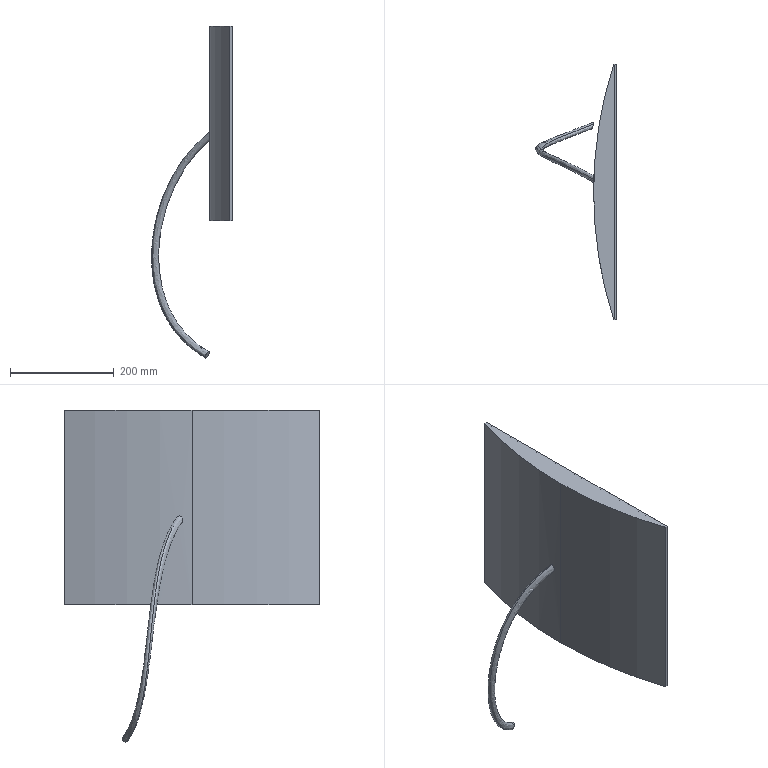Part | SolidWorks | features 3DProfileFeature 2, Extrusion 1, ICE 1, Sweep 1 | 1 solid | 15 faces | box 155.98 x 493 x 640.45 mm | volume 5277382 mm3 | plane 11 | spline 2 | cylinder 2 | commonest cylinder face diameters 1600 x2
STEP:
#1=CARTESIAN_POINT('',(-799.608,25.039,-32.684));
#2=VERTEX_POINT('',#1);
#3=CARTESIAN_POINT('',(-799.627,24.411,-16.43));
#4=VERTEX_POINT('',#3);
#5=CARTESIAN_POINT('',(-799.608,25.039,-32.684));
#6=CARTESIAN_POINT('',(-799.623,24.547,-32.674));
#7=CARTESIAN_POINT('',(-799.638,24.071,-32.597));
#8=CARTESIAN_POINT('',(-799.665,23.143,-32.327));
#9=CARTESIAN_POINT('',(-799.678,22.688,-32.13));
#10=CARTESIAN_POINT('',(-799.696,22.055,-31.769));
#11=CARTESIAN_POINT('',(-799.702,21.851,-31.637));
#12=CARTESIAN_POINT('',(-799.712,21.455,-31.352));
#13=CARTESIAN_POINT('',(-799.717,21.264,-31.198));
#14=CARTESIAN_POINT('',(-799.732,20.715,-30.713));
#15=CARTESIAN_POINT('',(-799.74,20.384,-30.358));
#16=CARTESIAN_POINT('',(-799.755,19.781,-29.594));
#17=CARTESIAN_POINT('',(-799.762,19.51,-29.183));
#18=CARTESIAN_POINT('',(-799.773,19.039,-28.334));
#19=CARTESIAN_POINT('',(-799.778,18.837,-27.894));
#20=CARTESIAN_POINT('',(-799.784,18.582,-27.209));
#21=CARTESIAN_POINT('',(-799.786,18.505,-26.976));
#22=CARTESIAN_POINT('',(-799.789,18.368,-26.508));
#23=CARTESIAN_POINT('',(-799.79,18.309,-26.273));
#24=CARTESIAN_POINT('',(-799.794,18.156,-25.563));
#25=CARTESIAN_POINT('',(-799.795,18.088,-25.085));
#26=CARTESIAN_POINT('',(-799.797,18.022,-24.117));
#27=CARTESIAN_POINT('',(-799.797,18.025,-23.624));
#28=CARTESIAN_POINT('',(-799.795,18.104,-22.659));
#29=CARTESIAN_POINT('',(-799.793,18.179,-22.183));
#30=CARTESIAN_POINT('',(-799.789,18.351,-21.481));
#31=CARTESIAN_POINT('',(-799.788,18.418,-21.248));
#32=CARTESIAN_POINT('',(-799.784,18.573,-20.788));
#33=CARTESIAN_POINT('',(-799.782,18.661,-20.558));
#34=CARTESIAN_POINT('',(-799.775,18.956,-19.887));
#35=CARTESIAN_POINT('',(-799.77,19.191,-19.463));
#36=CARTESIAN_POINT('',(-799.756,19.746,-18.666));
#37=CARTESIAN_POINT('',(-799.748,20.07,-18.29));
#38=CARTESIAN_POINT('',(-799.73,20.783,-17.636));
#39=CARTESIAN_POINT('',(-799.72,21.173,-17.351));
#40=CARTESIAN_POINT('',(-799.703,21.816,-16.999));
#41=CARTESIAN_POINT('',(-799.696,22.04,-16.894));
#42=CARTESIAN_POINT('',(-799.684,22.493,-16.717));
#43=CARTESIAN_POINT('',(-799.677,22.724,-16.644));
#44=CARTESIAN_POINT('',(-799.664,23.194,-16.529));
#45=CARTESIAN_POINT('',(-799.657,23.434,-16.487));
#46=CARTESIAN_POINT('',(-799.642,23.922,-16.434));
#47=CARTESIAN_POINT('',(-799.635,24.168,-16.424));
#48=CARTESIAN_POINT('',(-799.627,24.411,-16.43));
#49=B_SPLINE_CURVE_WITH_KNOTS('',3,(#5,#6,#7,#8,#9,#10,#11,#12,#13,#14,#15,#16,#17,#18,#19,#20,#21,#22,#23,#24,#25,#26,#27,#28,#29,#30,#31,#32,#33,#34,#35,#36,#37,#38,#39,#40,#41,#42,#43,#44,#45,#46,#47,#48),.UNSPECIFIED.,.F.,.F.,(4,2,2,2,2,2,2,2,2,2,2,2,2,2,2,2,2,2,2,2,2,4),(0.,0.001447,0.002894,0.003618,0.004341,0.005789,0.007236,0.008683,0.009407,0.01013,0.01158,0.01302,0.01447,0.0152,0.01592,0.01737,0.01881,0.02026,0.02098,0.02171,0.02243,0.02315),.UNSPECIFIED.);
#50=EDGE_CURVE('',#2,#4,#49,.T.);
#51=ORIENTED_EDGE('',*,*,#50,.T.);
#52=CARTESIAN_POINT('',(-808.512,124.272,-450.652));
#53=VERTEX_POINT('',#52);
#54=CARTESIAN_POINT('',(-799.627,24.411,-16.43));
#55=CARTESIAN_POINT('',(-804.722,27.259,-20.216));
#56=CARTESIAN_POINT('',(-809.675,29.945,-24.241));
#57=CARTESIAN_POINT('',(-831.242,41.331,-43.303));
#58=CARTESIAN_POINT('',(-846.186,48.341,-60.795));
#59=CARTESIAN_POINT('',(-871.819,59.64,-99.448));
#60=CARTESIAN_POINT('',(-882.507,63.928,-120.607));
#61=CARTESIAN_POINT('',(-899.096,70.859,-164.921));
#62=CARTESIAN_POINT('',(-904.996,73.508,-188.073));
#63=CARTESIAN_POINT('',(-911.604,78.299,-234.737));
#64=CARTESIAN_POINT('',(-912.321,80.444,-258.248));
#65=CARTESIAN_POINT('',(-908.19,85.248,-304.097));
#66=CARTESIAN_POINT('',(-903.345,87.902,-326.441));
#67=CARTESIAN_POINT('',(-887.526,94.67,-368.458));
#68=CARTESIAN_POINT('',(-876.545,98.783,-388.138));
#69=CARTESIAN_POINT('',(-847.769,109.451,-423.139));
#70=CARTESIAN_POINT('',(-829.967,116.01,-438.451));
#71=CARTESIAN_POINT('',(-808.512,124.272,-450.652));
#72=B_SPLINE_CURVE_WITH_KNOTS('',3,(#54,#55,#56,#57,#58,#59,#60,#61,#62,#63,#64,#65,#66,#67,#68,#69,#70,#71),.UNSPECIFIED.,.F.,.F.,(4,2,2,2,2,2,2,2,4),(0.08918,0.125,0.25,0.375,0.5,0.625,0.75,0.875,1.),.UNSPECIFIED.);
#73=EDGE_CURVE('',#4,#53,#72,.T.);
#74=ORIENTED_EDGE('',*,*,#73,.T.);
#75=CARTESIAN_POINT('',(-800.416,131.734,-441.656));
#76=VERTEX_POINT('',#75);
#77=CARTESIAN_POINT('',(-804.464,128.003,-446.154));
#78=DIRECTION('',(-0.8213,0.3311,0.4645));
#79=DIRECTION('',(0.5694,0.5248,0.6327));
#80=AXIS2_PLACEMENT_3D('',#77,#78,#79);
#81=CIRCLE('',#80,7.109);
#82=EDGE_CURVE('',#53,#76,#81,.T.);
#83=ORIENTED_EDGE('',*,*,#82,.T.);
#84=CARTESIAN_POINT('',(-799.608,25.039,-32.684));
#85=CARTESIAN_POINT('',(-803.249,27.142,-35.657));
#86=CARTESIAN_POINT('',(-806.805,29.16,-38.765));
#87=CARTESIAN_POINT('',(-825.692,39.703,-56.371));
#88=CARTESIAN_POINT('',(-839.388,46.723,-73.249));
#89=CARTESIAN_POINT('',(-862.835,58.561,-110.495));
#90=CARTESIAN_POINT('',(-872.581,63.381,-130.861));
#91=CARTESIAN_POINT('',(-887.671,71.722,-173.447));
#92=CARTESIAN_POINT('',(-893.02,75.241,-195.663));
#93=CARTESIAN_POINT('',(-898.915,81.744,-240.318));
#94=CARTESIAN_POINT('',(-899.46,84.72,-262.756));
#95=CARTESIAN_POINT('',(-895.258,90.915,-306.258));
#96=CARTESIAN_POINT('',(-890.509,94.135,-327.318));
#97=CARTESIAN_POINT('',(-875.251,101.738,-366.523));
#98=CARTESIAN_POINT('',(-864.752,106.121,-384.668));
#99=CARTESIAN_POINT('',(-837.484,117.041,-416.692));
#100=CARTESIAN_POINT('',(-820.713,123.579,-430.585));
#101=CARTESIAN_POINT('',(-800.416,131.734,-441.656));
#102=B_SPLINE_CURVE_WITH_KNOTS('',3,(#84,#85,#86,#87,#88,#89,#90,#91,#92,#93,#94,#95,#96,#97,#98,#99,#100,#101),.UNSPECIFIED.,.F.,.F.,(4,2,2,2,2,2,2,2,4),(0.09687,0.125,0.25,0.375,0.5,0.625,0.75,0.875,1.),.UNSPECIFIED.);
#103=EDGE_CURVE('',#2,#76,#102,.T.);
#104=ORIENTED_EDGE('',*,*,#103,.F.);
#105=EDGE_LOOP('',(#51,#74,#83,#104));
#106=FACE_OUTER_BOUND('',#105,.T.);
#107=CARTESIAN_POINT('',(-759.077,0.,-7.109));
#108=CARTESIAN_POINT('',(-777.726,12.299,-15.756));
#109=CARTESIAN_POINT('',(-794.858,22.49,-27.627));
#110=CARTESIAN_POINT('',(-825.692,39.703,-56.371));
#111=CARTESIAN_POINT('',(-839.388,46.723,-73.249));
#112=CARTESIAN_POINT('',(-862.835,58.561,-110.495));
#113=CARTESIAN_POINT('',(-872.581,63.381,-130.861));
#114=CARTESIAN_POINT('',(-887.671,71.722,-173.447));
#115=CARTESIAN_POINT('',(-893.02,75.241,-195.663));
#116=CARTESIAN_POINT('',(-898.915,81.744,-240.318));
#117=CARTESIAN_POINT('',(-899.46,84.72,-262.756));
#118=CARTESIAN_POINT('',(-895.258,90.915,-306.258));
#119=CARTESIAN_POINT('',(-890.509,94.135,-327.318));
#120=CARTESIAN_POINT('',(-875.251,101.738,-366.523));
#121=CARTESIAN_POINT('',(-864.752,106.121,-384.668));
#122=CARTESIAN_POINT('',(-837.484,117.041,-416.692));
#123=CARTESIAN_POINT('',(-820.713,123.579,-430.585));
#124=CARTESIAN_POINT('',(-800.416,131.734,-441.656));
#125=CARTESIAN_POINT('',(-759.077,14.218,-7.109));
#126=CARTESIAN_POINT('',(-778.229,26.518,-16.401));
#127=CARTESIAN_POINT('',(-795.775,36.636,-28.921));
#128=CARTESIAN_POINT('',(-827.363,53.635,-58.761));
#129=CARTESIAN_POINT('',(-841.41,60.52,-76.085));
#130=CARTESIAN_POINT('',(-865.677,72.042,-114.055));
#131=CARTESIAN_POINT('',(-875.9,76.678,-134.703));
#132=CARTESIAN_POINT('',(-892.018,84.529,-177.881));
#133=CARTESIAN_POINT('',(-897.911,87.735,-200.416));
#134=CARTESIAN_POINT('',(-904.625,93.542,-245.868));
#135=CARTESIAN_POINT('',(-905.433,96.143,-268.785));
#136=CARTESIAN_POINT('',(-901.239,101.734,-313.307));
#137=CARTESIAN_POINT('',(-896.235,104.731,-334.905));
#138=CARTESIAN_POINT('',(-879.972,112.146,-375.01));
#139=CARTESIAN_POINT('',(-868.721,116.564,-393.507));
#140=CARTESIAN_POINT('',(-839.746,127.746,-425.815));
#141=CARTESIAN_POINT('',(-822.035,134.503,-439.634));
#142=CARTESIAN_POINT('',(-800.904,142.884,-450.466));
#143=CARTESIAN_POINT('',(-759.077,14.218,7.109));
#144=CARTESIAN_POINT('',(-779.636,27.162,-2.182));
#145=CARTESIAN_POINT('',(-798.632,37.778,-14.965));
#146=CARTESIAN_POINT('',(-832.913,55.263,-45.692));
#147=CARTESIAN_POINT('',(-848.208,62.138,-63.631));
#148=CARTESIAN_POINT('',(-874.661,73.121,-103.007));
#149=CARTESIAN_POINT('',(-885.826,77.224,-124.449));
#150=CARTESIAN_POINT('',(-903.443,83.666,-169.355));
#151=CARTESIAN_POINT('',(-909.887,86.002,-192.826));
#152=CARTESIAN_POINT('',(-917.314,90.097,-240.287));
#153=CARTESIAN_POINT('',(-918.295,91.867,-264.277));
#154=CARTESIAN_POINT('',(-914.172,96.067,-311.146));
#155=CARTESIAN_POINT('',(-909.071,98.498,-334.029));
#156=CARTESIAN_POINT('',(-892.248,105.077,-376.945));
#157=CARTESIAN_POINT('',(-880.515,109.226,-396.976));
#158=CARTESIAN_POINT('',(-850.031,120.155,-432.262));
#159=CARTESIAN_POINT('',(-831.288,126.934,-447.5));
#160=CARTESIAN_POINT('',(-809.,135.421,-459.462));
#161=CARTESIAN_POINT('',(-759.077,0.,7.109));
#162=CARTESIAN_POINT('',(-779.134,12.944,-1.538));
#163=CARTESIAN_POINT('',(-797.715,23.632,-13.671));
#164=CARTESIAN_POINT('',(-831.242,41.331,-43.303));
#165=CARTESIAN_POINT('',(-846.186,48.341,-60.795));
#166=CARTESIAN_POINT('',(-871.819,59.64,-99.448));
#167=CARTESIAN_POINT('',(-882.507,63.928,-120.607));
#168=CARTESIAN_POINT('',(-899.096,70.859,-164.921));
#169=CARTESIAN_POINT('',(-904.996,73.508,-188.073));
#170=CARTESIAN_POINT('',(-911.604,78.299,-234.737));
#171=CARTESIAN_POINT('',(-912.321,80.444,-258.248));
#172=CARTESIAN_POINT('',(-908.19,85.248,-304.097));
#173=CARTESIAN_POINT('',(-903.345,87.902,-326.441));
#174=CARTESIAN_POINT('',(-887.526,94.67,-368.458));
#175=CARTESIAN_POINT('',(-876.545,98.783,-388.138));
#176=CARTESIAN_POINT('',(-847.769,109.451,-423.139));
#177=CARTESIAN_POINT('',(-829.967,116.01,-438.451));
#178=CARTESIAN_POINT('',(-808.512,124.272,-450.652));
#179=CARTESIAN_POINT('',(-759.077,-14.218,7.109));
#180=CARTESIAN_POINT('',(-778.631,-1.274,-0.8927));
#181=CARTESIAN_POINT('',(-796.798,9.486,-12.378));
#182=CARTESIAN_POINT('',(-829.57,27.398,-40.913));
#183=CARTESIAN_POINT('',(-844.163,34.545,-57.958));
#184=CARTESIAN_POINT('',(-868.977,46.159,-95.888));
#185=CARTESIAN_POINT('',(-879.188,50.631,-116.766));
#186=CARTESIAN_POINT('',(-894.749,58.052,-160.487));
#187=CARTESIAN_POINT('',(-900.105,61.014,-183.32));
#188=CARTESIAN_POINT('',(-905.894,66.501,-229.186));
#189=CARTESIAN_POINT('',(-906.348,69.021,-252.219));
#190=CARTESIAN_POINT('',(-902.209,74.429,-297.048));
#191=CARTESIAN_POINT('',(-897.619,77.307,-318.854));
#192=CARTESIAN_POINT('',(-882.805,84.263,-359.972));
#193=CARTESIAN_POINT('',(-872.576,88.34,-379.299));
#194=CARTESIAN_POINT('',(-845.507,98.747,-414.016));
#195=CARTESIAN_POINT('',(-828.645,105.086,-429.402));
#196=CARTESIAN_POINT('',(-808.025,113.123,-441.842));
#197=CARTESIAN_POINT('',(-759.077,-14.218,-7.109));
#198=CARTESIAN_POINT('',(-777.224,-1.919,-15.111));
#199=CARTESIAN_POINT('',(-793.941,8.344,-26.334));
#200=CARTESIAN_POINT('',(-824.02,25.771,-53.981));
#201=CARTESIAN_POINT('',(-837.366,32.927,-70.412));
#202=CARTESIAN_POINT('',(-859.993,45.08,-106.936));
#203=CARTESIAN_POINT('',(-869.262,50.085,-127.02));
#204=CARTESIAN_POINT('',(-883.324,58.915,-169.013));
#205=CARTESIAN_POINT('',(-888.129,62.747,-190.91));
#206=CARTESIAN_POINT('',(-893.205,69.946,-234.767));
#207=CARTESIAN_POINT('',(-893.486,73.297,-256.727));
#208=CARTESIAN_POINT('',(-889.277,80.096,-299.209));
#209=CARTESIAN_POINT('',(-884.782,83.54,-319.73));
#210=CARTESIAN_POINT('',(-870.53,91.331,-358.037));
#211=CARTESIAN_POINT('',(-860.783,95.678,-375.83));
#212=CARTESIAN_POINT('',(-835.222,106.337,-407.569));
#213=CARTESIAN_POINT('',(-819.392,112.655,-421.537));
#214=CARTESIAN_POINT('',(-799.929,120.585,-432.846));
#215=CARTESIAN_POINT('',(-759.077,0.,-7.109));
#216=CARTESIAN_POINT('',(-777.726,12.299,-15.756));
#217=CARTESIAN_POINT('',(-794.858,22.49,-27.627));
#218=CARTESIAN_POINT('',(-825.692,39.703,-56.371));
#219=CARTESIAN_POINT('',(-839.388,46.723,-73.249));
#220=CARTESIAN_POINT('',(-862.835,58.561,-110.495));
#221=CARTESIAN_POINT('',(-872.581,63.381,-130.861));
#222=CARTESIAN_POINT('',(-887.671,71.722,-173.447));
#223=CARTESIAN_POINT('',(-893.02,75.241,-195.663));
#224=CARTESIAN_POINT('',(-898.915,81.744,-240.318));
#225=CARTESIAN_POINT('',(-899.46,84.72,-262.756));
#226=CARTESIAN_POINT('',(-895.258,90.915,-306.258));
#227=CARTESIAN_POINT('',(-890.509,94.135,-327.318));
#228=CARTESIAN_POINT('',(-875.251,101.738,-366.523));
#229=CARTESIAN_POINT('',(-864.752,106.121,-384.668));
#230=CARTESIAN_POINT('',(-837.484,117.041,-416.692));
#231=CARTESIAN_POINT('',(-820.713,123.579,-430.585));
#232=CARTESIAN_POINT('',(-800.416,131.734,-441.656));
#233=(BOUNDED_SURFACE()B_SPLINE_SURFACE(3,3,((#107,#108,#109,#110,#111,#112,#113,#114,#115,#116,#117,#118,#119,#120,#121,#122,#123,#124),(#125,#126,#127,#128,#129,#130,#131,#132,#133,#134,#135,#136,#137,#138,#139,#140,#141,#142),(#143,#144,#145,#146,#147,#148,#149,#150,#151,#152,#153,#154,#155,#156,#157,#158,#159,#160),(#161,#162,#163,#164,#165,#166,#167,#168,#169,#170,#171,#172,#173,#174,#175,#176,#177,#178),(#179,#180,#181,#182,#183,#184,#185,#186,#187,#188,#189,#190,#191,#192,#193,#194,#195,#196),(#197,#198,#199,#200,#201,#202,#203,#204,#205,#206,#207,#208,#209,#210,#211,#212,#213,#214),(#215,#216,#217,#218,#219,#220,#221,#222,#223,#224,#225,#226,#227,#228,#229,#230,#231,#232)),.UNSPECIFIED.,.T.,.F.,.F.)B_SPLINE_SURFACE_WITH_KNOTS((4,3,4),(4,2,2,2,2,2,2,2,4),(0.,0.5,1.),(0.,0.125,0.25,0.375,0.5,0.625,0.75,0.875,1.),.UNSPECIFIED.)GEOMETRIC_REPRESENTATION_ITEM()RATIONAL_B_SPLINE_SURFACE(((1.,1.,1.,1.,1.,1.,1.,1.,1.,1.,1.,1.,1.,1.,1.,1.,1.,1.),(0.3333,0.3333,0.3333,0.3333,0.3333,0.3333,0.3333,0.3333,0.3333,0.3333,0.3333,0.3333,0.3333,0.3333,0.3333,0.3333,0.3333,0.3333),(0.3333,0.3333,0.3333,0.3333,0.3333,0.3333,0.3333,0.3333,0.3333,0.3333,0.3333,0.3333,0.3333,0.3333,0.3333,0.3333,0.3333,0.3333),(1.,1.,1.,1.,1.,1.,1.,1.,1.,1.,1.,1.,1.,1.,1.,1.,1.,1.),(0.3333,0.3333,0.3333,0.3333,0.3333,0.3333,0.3333,0.3333,0.3333,0.3333,0.3333,0.3333,0.3333,0.3333,0.3333,0.3333,0.3333,0.3333),(0.3333,0.3333,0.3333,0.3333,0.3333,0.3333,0.3333,0.3333,0.3333,0.3333,0.3333,0.3333,0.3333,0.3333,0.3333,0.3333,0.3333,0.3333),(1.,1.,1.,1.,1.,1.,1.,1.,1.,1.,1.,1.,1.,1.,1.,1.,1.,1.)))REPRESENTATION_ITEM('')SURFACE());
#234=ADVANCED_FACE('',(#106),#233,.F.);
#235=CARTESIAN_POINT('',(-800.,0.,188.));
#236=VERTEX_POINT('',#235);
#237=CARTESIAN_POINT('',(-761.077,-246.5,188.));
#238=VERTEX_POINT('',#237);
#239=CARTESIAN_POINT('',(0.,0.,188.));
#240=DIRECTION('',(0.,0.,1.));
#241=DIRECTION('',(1.,0.,0.));
#242=AXIS2_PLACEMENT_3D('',#239,#240,#241);
#243=CIRCLE('',#242,800.);
#244=EDGE_CURVE('',#236,#238,#243,.T.);
#245=ORIENTED_EDGE('',*,*,#244,.F.);
#246=CARTESIAN_POINT('',(-800.,0.,-188.));
#247=VERTEX_POINT('',#246);
#248=CARTESIAN_POINT('',(-800.,0.,188.));
#249=DIRECTION('',(0.,0.,-1.));
#250=VECTOR('',#249,1000.);
#251=LINE('',#248,#250);
#252=EDGE_CURVE('',#236,#247,#251,.T.);
#253=ORIENTED_EDGE('',*,*,#252,.T.);
#254=CARTESIAN_POINT('',(-761.077,-246.5,-188.));
#255=VERTEX_POINT('',#254);
#256=CARTESIAN_POINT('',(0.,0.,-188.));
#257=DIRECTION('',(0.,0.,1.));
#258=DIRECTION('',(1.,0.,0.));
#259=AXIS2_PLACEMENT_3D('',#256,#257,#258);
#260=CIRCLE('',#259,800.);
#261=EDGE_CURVE('',#247,#255,#260,.T.);
#262=ORIENTED_EDGE('',*,*,#261,.T.);
#263=CARTESIAN_POINT('',(-761.077,-246.5,188.));
#264=DIRECTION('',(0.,0.,-1.));
#265=VECTOR('',#264,1000.);
#266=LINE('',#263,#265);
#267=EDGE_CURVE('',#238,#255,#266,.T.);
#268=ORIENTED_EDGE('',*,*,#267,.F.);
#269=EDGE_LOOP('',(#245,#253,#262,#268));
#270=FACE_OUTER_BOUND('',#269,.T.);
#271=CARTESIAN_POINT('',(0.,0.,188.));
#272=DIRECTION('',(0.,0.,-1.));
#273=DIRECTION('',(-1.,0.,0.));
#274=AXIS2_PLACEMENT_3D('',#271,#272,#273);
#275=CYLINDRICAL_SURFACE('',#274,800.);
#276=ADVANCED_FACE('',(#270),#275,.T.);
#277=ORIENTED_EDGE('',*,*,#252,.F.);
#278=CARTESIAN_POINT('',(-761.077,246.5,188.));
#279=VERTEX_POINT('',#278);
#280=CARTESIAN_POINT('',(0.,0.,188.));
#281=DIRECTION('',(0.,0.,1.));
#282=DIRECTION('',(1.,0.,0.));
#283=AXIS2_PLACEMENT_3D('',#280,#281,#282);
#284=CIRCLE('',#283,800.);
#285=EDGE_CURVE('',#279,#236,#284,.T.);
#286=ORIENTED_EDGE('',*,*,#285,.F.);
#287=CARTESIAN_POINT('',(-761.077,246.5,-188.));
#288=VERTEX_POINT('',#287);
#289=CARTESIAN_POINT('',(-761.077,246.5,188.));
#290=DIRECTION('',(0.,0.,-1.));
#291=VECTOR('',#290,1000.);
#292=LINE('',#289,#291);
#293=EDGE_CURVE('',#279,#288,#292,.T.);
#294=ORIENTED_EDGE('',*,*,#293,.T.);
#295=CARTESIAN_POINT('',(0.,0.,-188.));
#296=DIRECTION('',(0.,0.,1.));
#297=DIRECTION('',(1.,0.,0.));
#298=AXIS2_PLACEMENT_3D('',#295,#296,#297);
#299=CIRCLE('',#298,800.);
#300=EDGE_CURVE('',#288,#247,#299,.T.);
#301=ORIENTED_EDGE('',*,*,#300,.T.);
#302=EDGE_LOOP('',(#277,#286,#294,#301));
#303=FACE_OUTER_BOUND('',#302,.T.);
#304=ORIENTED_EDGE('',*,*,#50,.F.);
#305=CARTESIAN_POINT('',(-799.627,24.411,-16.43));
#306=CARTESIAN_POINT('',(-799.62,24.653,-16.436));
#307=CARTESIAN_POINT('',(-799.613,24.893,-16.458));
#308=CARTESIAN_POINT('',(-799.598,25.371,-16.531));
#309=CARTESIAN_POINT('',(-799.59,25.611,-16.584));
#310=CARTESIAN_POINT('',(-799.567,26.313,-16.784));
#311=CARTESIAN_POINT('',(-799.552,26.759,-16.971));
#312=CARTESIAN_POINT('',(-799.531,27.396,-17.326));
#313=CARTESIAN_POINT('',(-799.524,27.604,-17.457));
#314=CARTESIAN_POINT('',(-799.51,28.,-17.736));
#315=CARTESIAN_POINT('',(-799.503,28.19,-17.885));
#316=CARTESIAN_POINT('',(-799.484,28.738,-18.361));
#317=CARTESIAN_POINT('',(-799.472,29.076,-18.717));
#318=CARTESIAN_POINT('',(-799.449,29.678,-19.476));
#319=CARTESIAN_POINT('',(-799.439,29.944,-19.879));
#320=CARTESIAN_POINT('',(-799.422,30.412,-20.729));
#321=CARTESIAN_POINT('',(-799.414,30.612,-21.176));
#322=CARTESIAN_POINT('',(-799.401,30.941,-22.084));
#323=CARTESIAN_POINT('',(-799.396,31.07,-22.549));
#324=CARTESIAN_POINT('',(-799.389,31.262,-23.499));
#325=CARTESIAN_POINT('',(-799.387,31.323,-23.985));
#326=CARTESIAN_POINT('',(-799.385,31.375,-24.947));
#327=CARTESIAN_POINT('',(-799.385,31.366,-25.428));
#328=CARTESIAN_POINT('',(-799.388,31.276,-26.389));
#329=CARTESIAN_POINT('',(-799.392,31.194,-26.874));
#330=CARTESIAN_POINT('',(-799.401,30.959,-27.81));
#331=CARTESIAN_POINT('',(-799.407,30.805,-28.264));
#332=CARTESIAN_POINT('',(-799.418,30.518,-28.924));
#333=CARTESIAN_POINT('',(-799.422,30.412,-29.14));
#334=CARTESIAN_POINT('',(-799.431,30.181,-29.564));
#335=CARTESIAN_POINT('',(-799.435,30.053,-29.773));
#336=CARTESIAN_POINT('',(-799.451,29.643,-30.378));
#337=CARTESIAN_POINT('',(-799.462,29.334,-30.75));
#338=CARTESIAN_POINT('',(-799.481,28.809,-31.253));
#339=CARTESIAN_POINT('',(-799.488,28.623,-31.412));
#340=CARTESIAN_POINT('',(-799.502,28.234,-31.706));
#341=CARTESIAN_POINT('',(-799.509,28.032,-31.84));
#342=CARTESIAN_POINT('',(-799.523,27.615,-32.081));
#343=CARTESIAN_POINT('',(-799.531,27.4,-32.187));
#344=CARTESIAN_POINT('',(-799.546,26.954,-32.372));
#345=CARTESIAN_POINT('',(-799.554,26.722,-32.451));
#346=CARTESIAN_POINT('',(-799.577,26.012,-32.637));
#347=CARTESIAN_POINT('',(-799.593,25.528,-32.694));
#348=CARTESIAN_POINT('',(-799.608,25.039,-32.684));
#349=B_SPLINE_CURVE_WITH_KNOTS('',3,(#305,#306,#307,#308,#309,#310,#311,#312,#313,#314,#315,#316,#317,#318,#319,#320,#321,#322,#323,#324,#325,#326,#327,#328,#329,#330,#331,#332,#333,#334,#335,#336,#337,#338,#339,#340,#341,#342,#343,#344,#345,#346,#347,#348),.UNSPECIFIED.,.F.,.F.,(4,2,2,2,2,2,2,2,2,2,2,2,2,2,2,2,2,2,2,2,2,4),(0.02315,0.02387,0.02459,0.02603,0.02675,0.02747,0.02891,0.03034,0.03178,0.03322,0.03466,0.0361,0.03753,0.03897,0.03969,0.04041,0.04185,0.04257,0.04329,0.04401,0.04472,0.04616),.UNSPECIFIED.);
#350=EDGE_CURVE('',#4,#2,#349,.T.);
#351=ORIENTED_EDGE('',*,*,#350,.F.);
#352=EDGE_LOOP('',(#304,#351));
#353=FACE_BOUND('',#352,.T.);
#354=CARTESIAN_POINT('',(0.,0.,188.));
#355=DIRECTION('',(0.,0.,-1.));
#356=DIRECTION('',(-1.,0.,0.));
#357=AXIS2_PLACEMENT_3D('',#354,#355,#356);
#358=CYLINDRICAL_SURFACE('',#357,800.);
#359=ADVANCED_FACE('',(#303,#353),#358,.T.);
#360=CARTESIAN_POINT('',(-756.077,246.5,-188.));
#361=VERTEX_POINT('',#360);
#362=CARTESIAN_POINT('',(0.,246.5,-188.));
#363=DIRECTION('',(-1.,0.,0.));
#364=VECTOR('',#363,1000.);
#365=LINE('',#362,#364);
#366=EDGE_CURVE('',#361,#288,#365,.T.);
#367=ORIENTED_EDGE('',*,*,#366,.T.);
#368=ORIENTED_EDGE('',*,*,#293,.F.);
#369=CARTESIAN_POINT('',(-756.077,246.5,188.));
#370=VERTEX_POINT('',#369);
#371=CARTESIAN_POINT('',(0.,246.5,188.));
#372=DIRECTION('',(-1.,0.,0.));
#373=VECTOR('',#372,1000.);
#374=LINE('',#371,#373);
#375=EDGE_CURVE('',#370,#279,#374,.T.);
#376=ORIENTED_EDGE('',*,*,#375,.F.);
#377=CARTESIAN_POINT('',(-756.077,246.5,188.));
#378=DIRECTION('',(0.,0.,-1.));
#379=VECTOR('',#378,1000.);
#380=LINE('',#377,#379);
#381=EDGE_CURVE('',#370,#361,#380,.T.);
#382=ORIENTED_EDGE('',*,*,#381,.T.);
#383=EDGE_LOOP('',(#367,#368,#376,#382));
#384=FACE_OUTER_BOUND('',#383,.T.);
#385=CARTESIAN_POINT('',(0.,246.5,188.));
#386=DIRECTION('',(0.,-1.,0.));
#387=DIRECTION('',(1.,0.,0.));
#388=AXIS2_PLACEMENT_3D('',#385,#386,#387);
#389=PLANE('',#388);
#390=ADVANCED_FACE('',(#384),#389,.F.);
#391=CARTESIAN_POINT('',(-756.077,-246.5,-188.));
#392=VERTEX_POINT('',#391);
#393=CARTESIAN_POINT('',(0.,-246.5,-188.));
#394=DIRECTION('',(-1.,0.,0.));
#395=VECTOR('',#394,1000.);
#396=LINE('',#393,#395);
#397=EDGE_CURVE('',#392,#255,#396,.T.);
#398=ORIENTED_EDGE('',*,*,#397,.F.);
#399=CARTESIAN_POINT('',(-756.077,-246.5,188.));
#400=VERTEX_POINT('',#399);
#401=CARTESIAN_POINT('',(-756.077,-246.5,188.));
#402=DIRECTION('',(0.,0.,-1.));
#403=VECTOR('',#402,1000.);
#404=LINE('',#401,#403);
#405=EDGE_CURVE('',#400,#392,#404,.T.);
#406=ORIENTED_EDGE('',*,*,#405,.F.);
#407=CARTESIAN_POINT('',(0.,-246.5,188.));
#408=DIRECTION('',(-1.,0.,0.));
#409=VECTOR('',#408,1000.);
#410=LINE('',#407,#409);
#411=EDGE_CURVE('',#400,#238,#410,.T.);
#412=ORIENTED_EDGE('',*,*,#411,.T.);
#413=ORIENTED_EDGE('',*,*,#267,.T.);
#414=EDGE_LOOP('',(#398,#406,#412,#413));
#415=FACE_OUTER_BOUND('',#414,.T.);
#416=CARTESIAN_POINT('',(0.,-246.5,188.));
#417=DIRECTION('',(0.,-1.,0.));
#418=DIRECTION('',(1.,0.,0.));
#419=AXIS2_PLACEMENT_3D('',#416,#417,#418);
#420=PLANE('',#419);
#421=ADVANCED_FACE('',(#415),#420,.T.);
#422=CARTESIAN_POINT('',(-756.077,-244.5,-186.));
#423=VERTEX_POINT('',#422);
#424=CARTESIAN_POINT('',(-756.077,244.5,-186.));
#425=VERTEX_POINT('',#424);
#426=CARTESIAN_POINT('',(-756.077,-244.5,-186.));
#427=DIRECTION('',(0.,1.,0.));
#428=VECTOR('',#427,1000.);
#429=LINE('',#426,#428);
#430=EDGE_CURVE('',#423,#425,#429,.T.);
#431=ORIENTED_EDGE('',*,*,#430,.F.);
#432=CARTESIAN_POINT('',(-756.077,-244.5,186.));
#433=VERTEX_POINT('',#432);
#434=CARTESIAN_POINT('',(-756.077,-244.5,186.));
#435=DIRECTION('',(0.,0.,-1.));
#436=VECTOR('',#435,1000.);
#437=LINE('',#434,#436);
#438=EDGE_CURVE('',#433,#423,#437,.T.);
#439=ORIENTED_EDGE('',*,*,#438,.F.);
#440=CARTESIAN_POINT('',(-756.077,244.5,186.));
#441=VERTEX_POINT('',#440);
#442=CARTESIAN_POINT('',(-756.077,244.5,186.));
#443=DIRECTION('',(0.,-1.,0.));
#444=VECTOR('',#443,1000.);
#445=LINE('',#442,#444);
#446=EDGE_CURVE('',#441,#433,#445,.T.);
#447=ORIENTED_EDGE('',*,*,#446,.F.);
#448=CARTESIAN_POINT('',(-756.077,244.5,-186.));
#449=DIRECTION('',(0.,0.,1.));
#450=VECTOR('',#449,1000.);
#451=LINE('',#448,#450);
#452=EDGE_CURVE('',#425,#441,#451,.T.);
#453=ORIENTED_EDGE('',*,*,#452,.F.);
#454=EDGE_LOOP('',(#431,#439,#447,#453));
#455=FACE_BOUND('',#454,.T.);
#456=CARTESIAN_POINT('',(-756.077,0.,-188.));
#457=DIRECTION('',(0.,1.,0.));
#458=VECTOR('',#457,1000.);
#459=LINE('',#456,#458);
#460=EDGE_CURVE('',#392,#361,#459,.T.);
#461=ORIENTED_EDGE('',*,*,#460,.T.);
#462=ORIENTED_EDGE('',*,*,#381,.F.);
#463=CARTESIAN_POINT('',(-756.077,0.,188.));
#464=DIRECTION('',(0.,1.,0.));
#465=VECTOR('',#464,1000.);
#466=LINE('',#463,#465);
#467=EDGE_CURVE('',#400,#370,#466,.T.);
#468=ORIENTED_EDGE('',*,*,#467,.F.);
#469=ORIENTED_EDGE('',*,*,#405,.T.);
#470=EDGE_LOOP('',(#461,#462,#468,#469));
#471=FACE_OUTER_BOUND('',#470,.T.);
#472=CARTESIAN_POINT('',(-756.077,0.,188.));
#473=DIRECTION('',(-1.,0.,0.));
#474=DIRECTION('',(0.,-1.,0.));
#475=AXIS2_PLACEMENT_3D('',#472,#473,#474);
#476=PLANE('',#475);
#477=ADVANCED_FACE('',(#455,#471),#476,.F.);
#478=ORIENTED_EDGE('',*,*,#375,.T.);
#479=ORIENTED_EDGE('',*,*,#285,.T.);
#480=ORIENTED_EDGE('',*,*,#244,.T.);
#481=ORIENTED_EDGE('',*,*,#411,.F.);
#482=ORIENTED_EDGE('',*,*,#467,.T.);
#483=EDGE_LOOP('',(#478,#479,#480,#481,#482));
#484=FACE_OUTER_BOUND('',#483,.T.);
#485=CARTESIAN_POINT('',(0.,0.,188.));
#486=DIRECTION('',(0.,0.,1.));
#487=DIRECTION('',(1.,0.,0.));
#488=AXIS2_PLACEMENT_3D('',#485,#486,#487);
#489=PLANE('',#488);
#490=ADVANCED_FACE('',(#484),#489,.T.);
#491=ORIENTED_EDGE('',*,*,#366,.F.);
#492=ORIENTED_EDGE('',*,*,#460,.F.);
#493=ORIENTED_EDGE('',*,*,#397,.T.);
#494=ORIENTED_EDGE('',*,*,#261,.F.);
#495=ORIENTED_EDGE('',*,*,#300,.F.);
#496=EDGE_LOOP('',(#491,#492,#493,#494,#495));
#497=FACE_OUTER_BOUND('',#496,.T.);
#498=CARTESIAN_POINT('',(0.,0.,-188.));
#499=DIRECTION('',(0.,0.,1.));
#500=DIRECTION('',(1.,0.,0.));
#501=AXIS2_PLACEMENT_3D('',#498,#499,#500);
#502=PLANE('',#501);
#503=ADVANCED_FACE('',(#497),#502,.F.);
#504=ORIENTED_EDGE('',*,*,#438,.T.);
#505=CARTESIAN_POINT('',(-759.077,-244.5,-186.));
#506=VERTEX_POINT('',#505);
#507=CARTESIAN_POINT('',(-759.077,-244.5,-186.));
#508=DIRECTION('',(1.,0.,0.));
#509=VECTOR('',#508,1000.);
#510=LINE('',#507,#509);
#511=EDGE_CURVE('',#506,#423,#510,.T.);
#512=ORIENTED_EDGE('',*,*,#511,.F.);
#513=CARTESIAN_POINT('',(-759.077,-244.5,186.));
#514=VERTEX_POINT('',#513);
#515=CARTESIAN_POINT('',(-759.077,-244.5,186.));
#516=DIRECTION('',(0.,0.,-1.));
#517=VECTOR('',#516,1000.);
#518=LINE('',#515,#517);
#519=EDGE_CURVE('',#514,#506,#518,.T.);
#520=ORIENTED_EDGE('',*,*,#519,.F.);
#521=CARTESIAN_POINT('',(-759.077,-244.5,186.));
#522=DIRECTION('',(1.,0.,0.));
#523=VECTOR('',#522,1000.);
#524=LINE('',#521,#523);
#525=EDGE_CURVE('',#514,#433,#524,.T.);
#526=ORIENTED_EDGE('',*,*,#525,.T.);
#527=EDGE_LOOP('',(#504,#512,#520,#526));
#528=FACE_OUTER_BOUND('',#527,.T.);
#529=CARTESIAN_POINT('',(-759.077,-244.5,186.));
#530=DIRECTION('',(0.,-1.,0.));
#531=DIRECTION('',(0.,0.,-1.));
#532=AXIS2_PLACEMENT_3D('',#529,#530,#531);
#533=PLANE('',#532);
#534=ADVANCED_FACE('',(#528),#533,.F.);
#535=ORIENTED_EDGE('',*,*,#446,.T.);
#536=ORIENTED_EDGE('',*,*,#525,.F.);
#537=CARTESIAN_POINT('',(-759.077,244.5,186.));
#538=VERTEX_POINT('',#537);
#539=CARTESIAN_POINT('',(-759.077,244.5,186.));
#540=DIRECTION('',(0.,-1.,0.));
#541=VECTOR('',#540,1000.);
#542=LINE('',#539,#541);
#543=EDGE_CURVE('',#538,#514,#542,.T.);
#544=ORIENTED_EDGE('',*,*,#543,.F.);
#545=CARTESIAN_POINT('',(-759.077,244.5,186.));
#546=DIRECTION('',(1.,0.,0.));
#547=VECTOR('',#546,1000.);
#548=LINE('',#545,#547);
#549=EDGE_CURVE('',#538,#441,#548,.T.);
#550=ORIENTED_EDGE('',*,*,#549,.T.);
#551=EDGE_LOOP('',(#535,#536,#544,#550));
#552=FACE_OUTER_BOUND('',#551,.T.);
#553=CARTESIAN_POINT('',(-759.077,244.5,186.));
#554=DIRECTION('',(0.,0.,1.));
#555=DIRECTION('',(1.,0.,0.));
#556=AXIS2_PLACEMENT_3D('',#553,#554,#555);
#557=PLANE('',#556);
#558=ADVANCED_FACE('',(#552),#557,.F.);
#559=ORIENTED_EDGE('',*,*,#452,.T.);
#560=ORIENTED_EDGE('',*,*,#549,.F.);
#561=CARTESIAN_POINT('',(-759.077,244.5,-186.));
#562=VERTEX_POINT('',#561);
#563=CARTESIAN_POINT('',(-759.077,244.5,-186.));
#564=DIRECTION('',(0.,0.,1.));
#565=VECTOR('',#564,1000.);
#566=LINE('',#563,#565);
#567=EDGE_CURVE('',#562,#538,#566,.T.);
#568=ORIENTED_EDGE('',*,*,#567,.F.);
#569=CARTESIAN_POINT('',(-759.077,244.5,-186.));
#570=DIRECTION('',(1.,0.,0.));
#571=VECTOR('',#570,1000.);
#572=LINE('',#569,#571);
#573=EDGE_CURVE('',#562,#425,#572,.T.);
#574=ORIENTED_EDGE('',*,*,#573,.T.);
#575=EDGE_LOOP('',(#559,#560,#568,#574));
#576=FACE_OUTER_BOUND('',#575,.T.);
#577=CARTESIAN_POINT('',(-759.077,244.5,-186.));
#578=DIRECTION('',(0.,1.,0.));
#579=DIRECTION('',(0.,0.,1.));
#580=AXIS2_PLACEMENT_3D('',#577,#578,#579);
#581=PLANE('',#580);
#582=ADVANCED_FACE('',(#576),#581,.F.);
#583=ORIENTED_EDGE('',*,*,#430,.T.);
#584=ORIENTED_EDGE('',*,*,#573,.F.);
#585=CARTESIAN_POINT('',(-759.077,-244.5,-186.));
#586=DIRECTION('',(0.,1.,0.));
#587=VECTOR('',#586,1000.);
#588=LINE('',#585,#587);
#589=EDGE_CURVE('',#506,#562,#588,.T.);
#590=ORIENTED_EDGE('',*,*,#589,.F.);
#591=ORIENTED_EDGE('',*,*,#511,.T.);
#592=EDGE_LOOP('',(#583,#584,#590,#591));
#593=FACE_OUTER_BOUND('',#592,.T.);
#594=CARTESIAN_POINT('',(-759.077,-244.5,-186.));
#595=DIRECTION('',(0.,0.,-1.));
#596=DIRECTION('',(-1.,0.,0.));
#597=AXIS2_PLACEMENT_3D('',#594,#595,#596);
#598=PLANE('',#597);
#599=ADVANCED_FACE('',(#593),#598,.F.);
#600=ORIENTED_EDGE('',*,*,#519,.T.);
#601=ORIENTED_EDGE('',*,*,#589,.T.);
#602=ORIENTED_EDGE('',*,*,#567,.T.);
#603=ORIENTED_EDGE('',*,*,#543,.T.);
#604=EDGE_LOOP('',(#600,#601,#602,#603));
#605=FACE_OUTER_BOUND('',#604,.T.);
#606=CARTESIAN_POINT('',(-759.077,0.,0.));
#607=DIRECTION('',(1.,0.,0.));
#608=DIRECTION('',(0.,0.,-1.));
#609=AXIS2_PLACEMENT_3D('',#606,#607,#608);
#610=PLANE('',#609);
#611=ADVANCED_FACE('',(#605),#610,.T.);
#612=ORIENTED_EDGE('',*,*,#73,.F.);
#613=ORIENTED_EDGE('',*,*,#350,.T.);
#614=ORIENTED_EDGE('',*,*,#103,.T.);
#615=CARTESIAN_POINT('',(-804.464,128.003,-446.154));
#616=DIRECTION('',(-0.8213,0.3311,0.4645));
#617=DIRECTION('',(0.5694,0.5248,0.6327));
#618=AXIS2_PLACEMENT_3D('',#615,#616,#617);
#619=CIRCLE('',#618,7.109);
#620=EDGE_CURVE('',#76,#53,#619,.T.);
#621=ORIENTED_EDGE('',*,*,#620,.T.);
#622=EDGE_LOOP('',(#612,#613,#614,#621));
#623=FACE_OUTER_BOUND('',#622,.T.);
#624=CARTESIAN_POINT('',(-759.077,0.,-7.109));
#625=CARTESIAN_POINT('',(-777.726,12.299,-15.756));
#626=CARTESIAN_POINT('',(-794.858,22.49,-27.627));
#627=CARTESIAN_POINT('',(-825.692,39.703,-56.371));
#628=CARTESIAN_POINT('',(-839.388,46.723,-73.249));
#629=CARTESIAN_POINT('',(-862.835,58.561,-110.495));
#630=CARTESIAN_POINT('',(-872.581,63.381,-130.861));
#631=CARTESIAN_POINT('',(-887.671,71.722,-173.447));
#632=CARTESIAN_POINT('',(-893.02,75.241,-195.663));
#633=CARTESIAN_POINT('',(-898.915,81.744,-240.318));
#634=CARTESIAN_POINT('',(-899.46,84.72,-262.756));
#635=CARTESIAN_POINT('',(-895.258,90.915,-306.258));
#636=CARTESIAN_POINT('',(-890.509,94.135,-327.318));
#637=CARTESIAN_POINT('',(-875.251,101.738,-366.523));
#638=CARTESIAN_POINT('',(-864.752,106.121,-384.668));
#639=CARTESIAN_POINT('',(-837.484,117.041,-416.692));
#640=CARTESIAN_POINT('',(-820.713,123.579,-430.585));
#641=CARTESIAN_POINT('',(-800.416,131.734,-441.656));
#642=CARTESIAN_POINT('',(-759.077,14.218,-7.109));
#643=CARTESIAN_POINT('',(-778.229,26.518,-16.401));
#644=CARTESIAN_POINT('',(-795.775,36.636,-28.921));
#645=CARTESIAN_POINT('',(-827.363,53.635,-58.761));
#646=CARTESIAN_POINT('',(-841.41,60.52,-76.085));
#647=CARTESIAN_POINT('',(-865.677,72.042,-114.055));
#648=CARTESIAN_POINT('',(-875.9,76.678,-134.703));
#649=CARTESIAN_POINT('',(-892.018,84.529,-177.881));
#650=CARTESIAN_POINT('',(-897.911,87.735,-200.416));
#651=CARTESIAN_POINT('',(-904.625,93.542,-245.868));
#652=CARTESIAN_POINT('',(-905.433,96.143,-268.785));
#653=CARTESIAN_POINT('',(-901.239,101.734,-313.307));
#654=CARTESIAN_POINT('',(-896.235,104.731,-334.905));
#655=CARTESIAN_POINT('',(-879.972,112.146,-375.01));
#656=CARTESIAN_POINT('',(-868.721,116.564,-393.507));
#657=CARTESIAN_POINT('',(-839.746,127.746,-425.815));
#658=CARTESIAN_POINT('',(-822.035,134.503,-439.634));
#659=CARTESIAN_POINT('',(-800.904,142.884,-450.466));
#660=CARTESIAN_POINT('',(-759.077,14.218,7.109));
#661=CARTESIAN_POINT('',(-779.636,27.162,-2.182));
#662=CARTESIAN_POINT('',(-798.632,37.778,-14.965));
#663=CARTESIAN_POINT('',(-832.913,55.263,-45.692));
#664=CARTESIAN_POINT('',(-848.208,62.138,-63.631));
#665=CARTESIAN_POINT('',(-874.661,73.121,-103.007));
#666=CARTESIAN_POINT('',(-885.826,77.224,-124.449));
#667=CARTESIAN_POINT('',(-903.443,83.666,-169.355));
#668=CARTESIAN_POINT('',(-909.887,86.002,-192.826));
#669=CARTESIAN_POINT('',(-917.314,90.097,-240.287));
#670=CARTESIAN_POINT('',(-918.295,91.867,-264.277));
#671=CARTESIAN_POINT('',(-914.172,96.067,-311.146));
#672=CARTESIAN_POINT('',(-909.071,98.498,-334.029));
#673=CARTESIAN_POINT('',(-892.248,105.077,-376.945));
#674=CARTESIAN_POINT('',(-880.515,109.226,-396.976));
#675=CARTESIAN_POINT('',(-850.031,120.155,-432.262));
#676=CARTESIAN_POINT('',(-831.288,126.934,-447.5));
#677=CARTESIAN_POINT('',(-809.,135.421,-459.462));
#678=CARTESIAN_POINT('',(-759.077,0.,7.109));
#679=CARTESIAN_POINT('',(-779.134,12.944,-1.538));
#680=CARTESIAN_POINT('',(-797.715,23.632,-13.671));
#681=CARTESIAN_POINT('',(-831.242,41.331,-43.303));
#682=CARTESIAN_POINT('',(-846.186,48.341,-60.795));
#683=CARTESIAN_POINT('',(-871.819,59.64,-99.448));
#684=CARTESIAN_POINT('',(-882.507,63.928,-120.607));
#685=CARTESIAN_POINT('',(-899.096,70.859,-164.921));
#686=CARTESIAN_POINT('',(-904.996,73.508,-188.073));
#687=CARTESIAN_POINT('',(-911.604,78.299,-234.737));
#688=CARTESIAN_POINT('',(-912.321,80.444,-258.248));
#689=CARTESIAN_POINT('',(-908.19,85.248,-304.097));
#690=CARTESIAN_POINT('',(-903.345,87.902,-326.441));
#691=CARTESIAN_POINT('',(-887.526,94.67,-368.458));
#692=CARTESIAN_POINT('',(-876.545,98.783,-388.138));
#693=CARTESIAN_POINT('',(-847.769,109.451,-423.139));
#694=CARTESIAN_POINT('',(-829.967,116.01,-438.451));
#695=CARTESIAN_POINT('',(-808.512,124.272,-450.652));
#696=CARTESIAN_POINT('',(-759.077,-14.218,7.109));
#697=CARTESIAN_POINT('',(-778.631,-1.274,-0.8927));
#698=CARTESIAN_POINT('',(-796.798,9.486,-12.378));
#699=CARTESIAN_POINT('',(-829.57,27.398,-40.913));
#700=CARTESIAN_POINT('',(-844.163,34.545,-57.958));
#701=CARTESIAN_POINT('',(-868.977,46.159,-95.888));
#702=CARTESIAN_POINT('',(-879.188,50.631,-116.766));
#703=CARTESIAN_POINT('',(-894.749,58.052,-160.487));
#704=CARTESIAN_POINT('',(-900.105,61.014,-183.32));
#705=CARTESIAN_POINT('',(-905.894,66.501,-229.186));
#706=CARTESIAN_POINT('',(-906.348,69.021,-252.219));
#707=CARTESIAN_POINT('',(-902.209,74.429,-297.048));
#708=CARTESIAN_POINT('',(-897.619,77.307,-318.854));
#709=CARTESIAN_POINT('',(-882.805,84.263,-359.972));
#710=CARTESIAN_POINT('',(-872.576,88.34,-379.299));
#711=CARTESIAN_POINT('',(-845.507,98.747,-414.016));
#712=CARTESIAN_POINT('',(-828.645,105.086,-429.402));
#713=CARTESIAN_POINT('',(-808.025,113.123,-441.842));
#714=CARTESIAN_POINT('',(-759.077,-14.218,-7.109));
#715=CARTESIAN_POINT('',(-777.224,-1.919,-15.111));
#716=CARTESIAN_POINT('',(-793.941,8.344,-26.334));
#717=CARTESIAN_POINT('',(-824.02,25.771,-53.981));
#718=CARTESIAN_POINT('',(-837.366,32.927,-70.412));
#719=CARTESIAN_POINT('',(-859.993,45.08,-106.936));
#720=CARTESIAN_POINT('',(-869.262,50.085,-127.02));
#721=CARTESIAN_POINT('',(-883.324,58.915,-169.013));
#722=CARTESIAN_POINT('',(-888.129,62.747,-190.91));
#723=CARTESIAN_POINT('',(-893.205,69.946,-234.767));
#724=CARTESIAN_POINT('',(-893.486,73.297,-256.727));
#725=CARTESIAN_POINT('',(-889.277,80.096,-299.209));
#726=CARTESIAN_POINT('',(-884.782,83.54,-319.73));
#727=CARTESIAN_POINT('',(-870.53,91.331,-358.037));
#728=CARTESIAN_POINT('',(-860.783,95.678,-375.83));
#729=CARTESIAN_POINT('',(-835.222,106.337,-407.569));
#730=CARTESIAN_POINT('',(-819.392,112.655,-421.537));
#731=CARTESIAN_POINT('',(-799.929,120.585,-432.846));
#732=CARTESIAN_POINT('',(-759.077,0.,-7.109));
#733=CARTESIAN_POINT('',(-777.726,12.299,-15.756));
#734=CARTESIAN_POINT('',(-794.858,22.49,-27.627));
#735=CARTESIAN_POINT('',(-825.692,39.703,-56.371));
#736=CARTESIAN_POINT('',(-839.388,46.723,-73.249));
#737=CARTESIAN_POINT('',(-862.835,58.561,-110.495));
#738=CARTESIAN_POINT('',(-872.581,63.381,-130.861));
#739=CARTESIAN_POINT('',(-887.671,71.722,-173.447));
#740=CARTESIAN_POINT('',(-893.02,75.241,-195.663));
#741=CARTESIAN_POINT('',(-898.915,81.744,-240.318));
#742=CARTESIAN_POINT('',(-899.46,84.72,-262.756));
#743=CARTESIAN_POINT('',(-895.258,90.915,-306.258));
#744=CARTESIAN_POINT('',(-890.509,94.135,-327.318));
#745=CARTESIAN_POINT('',(-875.251,101.738,-366.523));
#746=CARTESIAN_POINT('',(-864.752,106.121,-384.668));
#747=CARTESIAN_POINT('',(-837.484,117.041,-416.692));
#748=CARTESIAN_POINT('',(-820.713,123.579,-430.585));
#749=CARTESIAN_POINT('',(-800.416,131.734,-441.656));
#750=(BOUNDED_SURFACE()B_SPLINE_SURFACE(3,3,((#624,#625,#626,#627,#628,#629,#630,#631,#632,#633,#634,#635,#636,#637,#638,#639,#640,#641),(#642,#643,#644,#645,#646,#647,#648,#649,#650,#651,#652,#653,#654,#655,#656,#657,#658,#659),(#660,#661,#662,#663,#664,#665,#666,#667,#668,#669,#670,#671,#672,#673,#674,#675,#676,#677),(#678,#679,#680,#681,#682,#683,#684,#685,#686,#687,#688,#689,#690,#691,#692,#693,#694,#695),(#696,#697,#698,#699,#700,#701,#702,#703,#704,#705,#706,#707,#708,#709,#710,#711,#712,#713),(#714,#715,#716,#717,#718,#719,#720,#721,#722,#723,#724,#725,#726,#727,#728,#729,#730,#731),(#732,#733,#734,#735,#736,#737,#738,#739,#740,#741,#742,#743,#744,#745,#746,#747,#748,#749)),.UNSPECIFIED.,.T.,.F.,.T.)B_SPLINE_SURFACE_WITH_KNOTS((4,3,4),(4,2,2,2,2,2,2,2,4),(0.,0.5,1.),(0.,0.125,0.25,0.375,0.5,0.625,0.75,0.875,1.),.UNSPECIFIED.)GEOMETRIC_REPRESENTATION_ITEM()RATIONAL_B_SPLINE_SURFACE(((1.,1.,1.,1.,1.,1.,1.,1.,1.,1.,1.,1.,1.,1.,1.,1.,1.,1.),(0.3333,0.3333,0.3333,0.3333,0.3333,0.3333,0.3333,0.3333,0.3333,0.3333,0.3333,0.3333,0.3333,0.3333,0.3333,0.3333,0.3333,0.3333),(0.3333,0.3333,0.3333,0.3333,0.3333,0.3333,0.3333,0.3333,0.3333,0.3333,0.3333,0.3333,0.3333,0.3333,0.3333,0.3333,0.3333,0.3333),(1.,1.,1.,1.,1.,1.,1.,1.,1.,1.,1.,1.,1.,1.,1.,1.,1.,1.),(0.3333,0.3333,0.3333,0.3333,0.3333,0.3333,0.3333,0.3333,0.3333,0.3333,0.3333,0.3333,0.3333,0.3333,0.3333,0.3333,0.3333,0.3333),(0.3333,0.3333,0.3333,0.3333,0.3333,0.3333,0.3333,0.3333,0.3333,0.3333,0.3333,0.3333,0.3333,0.3333,0.3333,0.3333,0.3333,0.3333),(1.,1.,1.,1.,1.,1.,1.,1.,1.,1.,1.,1.,1.,1.,1.,1.,1.,1.)))REPRESENTATION_ITEM('')SURFACE());
#751=ADVANCED_FACE('',(#623),#750,.F.);
#752=ORIENTED_EDGE('',*,*,#620,.F.);
#753=ORIENTED_EDGE('',*,*,#82,.F.);
#754=EDGE_LOOP('',(#752,#753));
#755=FACE_OUTER_BOUND('',#754,.T.);
#756=CARTESIAN_POINT('',(-804.464,128.003,-446.154));
#757=DIRECTION('',(-0.8213,0.3311,0.4645));
#758=DIRECTION('',(0.5694,0.5248,0.6327));
#759=AXIS2_PLACEMENT_3D('',#756,#757,#758);
#760=PLANE('',#759);
#761=ADVANCED_FACE('',(#755),#760,.F.);
#762=CLOSED_SHELL('',(#234,#276,#359,#390,#421,#477,#490,#503,#534,#558,#582,#599,#611,#751,#761));
#763=MANIFOLD_SOLID_BREP('',#762);
#764=CARTESIAN_POINT('',(0.,0.,0.));
#765=DIRECTION('',(0.,0.,1.));
#766=DIRECTION('',(1.,0.,0.));
#767=AXIS2_PLACEMENT_3D('',#764,#765,#766);
#768=(LENGTH_UNIT()NAMED_UNIT(*)SI_UNIT(.MILLI.,.METRE.));
#769=UNCERTAINTY_MEASURE_WITH_UNIT(LENGTH_MEASURE(0.00001),#768,'','');
#770=(NAMED_UNIT(*)PLANE_ANGLE_UNIT()SI_UNIT($,.RADIAN.));
#771=(NAMED_UNIT(*)SI_UNIT($,.STERADIAN.)SOLID_ANGLE_UNIT());
#772=(GEOMETRIC_REPRESENTATION_CONTEXT(3)GLOBAL_UNCERTAINTY_ASSIGNED_CONTEXT((#769))GLOBAL_UNIT_ASSIGNED_CONTEXT((#768,#770,#771))REPRESENTATION_CONTEXT('',''));
#773=ADVANCED_BREP_SHAPE_REPRESENTATION('',(#763,#767),#772);